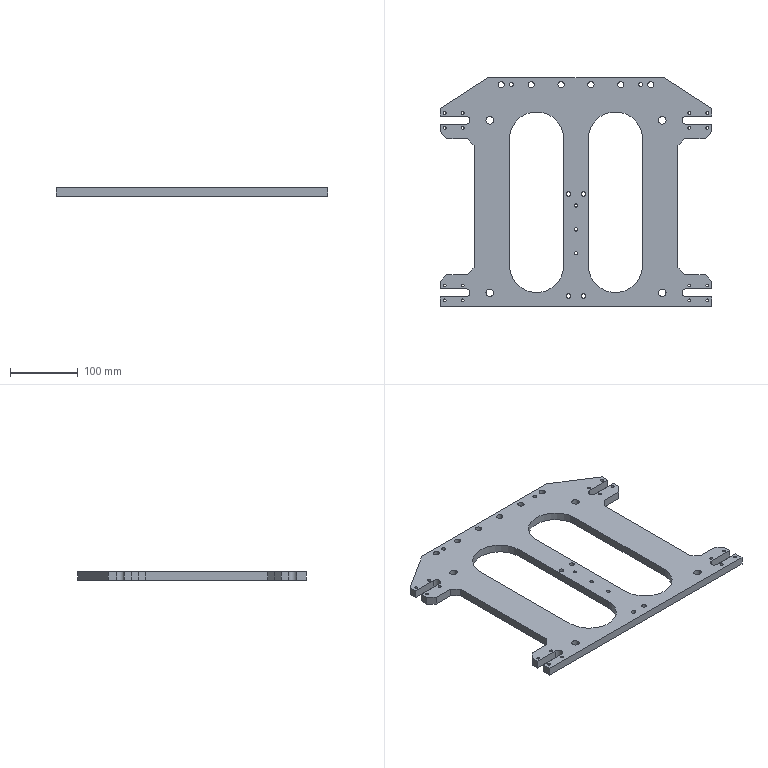NC program | NX | posted with a generic post | part box 400 x 336 x 12 mm
Lines 2735 to 3199 of 3199:
(ZLEVEL_PROFILE_COPY , TOOL : D10JING)
N5420 T09 M6
N5422 G54
N5424 G17 G0 G90 X-207.793 Y129.266 S5000 M3
N5426 G43 Z80. H9
N5428 Z-9.
N5430 G94 G1 Z-12. F1200.
N5432 X-203.703 Y127.158
N5434 G3 X-202.704 Y127.206 R1.
N5436 G1 X-132.704 Y172.206
N5438 G2 X-130. Y173. R5.
N5440 G1 X130.
N5442 G2 X132.704 Y172.206 R5.
N5444 G1 X202.704 Y127.206
N5446 G3 X203.703 Y127.158 R1.
N5448 G1 X207.793 Y129.266
N5450 Z-9.
N5452 G0 Z80.
N5454 X203.167 Y-177.485
N5456 Z-9.
N5458 G1 Z-12.
N5460 X200.866 Y-173.5
N5462 G3 X200. Y-173. R1.
N5464 G1 X-200.
N5466 G3 X-200.866 Y-173.5 R1.
N5468 G1 X-203.167 Y-177.485
N5470 Z-9.
N5472 G0 Z80.
N5474 M5
(ZLEVEL_PROFILE_COPY_COPY_1 , TOOL : D6)
N5476 T06 M6
N5478 G54
N5480 G17 G0 G90 X-94.939 Y78.263 S5000 M3
N5482 G43 Z80. H6
N5484 Z-8.9
N5486 G94 G1 Z-11.9 F1200.
N5488 G3 X-95. Y78. R0.6
N5490 G1 Y-108.
N5492 G3 X-58. Y-145. R37.
N5494 X-21. Y-108. R37.
N5496 G1 Y78.
N5498 G3 X-58. Y115. R37.
N5500 X-95. Y78. R37.
N5502 X-94.94 Y77.738 R0.6
N5504 G1 Z-8.9
N5506 G0 Z80.
N5508 X94.939 Y-108.263
N5510 Z-8.9
N5512 G1 Z-11.9
N5514 G3 X95. Y-108. R0.6
N5516 G1 Y78.
N5518 G3 X58. Y115. R37.
N5520 X21. Y78. R37.
N5522 G1 Y-108.
N5524 G3 X58. Y-145. R37.
N5526 X95. Y-108. R37.
N5528 X94.94 Y-107.738 R0.6
N5530 G1 Z-8.9
N5532 G0 Z80.
N5534 M5
(ZLEVEL_PROFILE_COPY_COPY , TOOL : D6A45)
N5536 T07 M6
N5538 G54
N5540 G17 G0 G90 X-194.483 Y116.5 S7500 M3
N5542 G43 Z80. H7
N5544 Z3.
N5546 G94 G1 Z-1. F1200.
N5548 G3 X-193.3 Y115.317 R1.183
N5550 X-194.483 Y116.5 R-1.183
N5552 X-194.183 Y115.98 R0.6
N5554 G1 Z2.
N5556 G0 Z80.
N5558 X-94.753 Y158.848
N5560 Z2.
N5562 G1 Z-1.
N5564 X-94.48 Y159.783
N5566 G3 X-95. Y160.083 R0.6
N5568 X-97.083 Y158. R2.083
N5570 X-95. Y160.083 R-2.083
N5572 X-95.52 Y159.783 R0.6
N5574 G1 X-95.247 Y158.848
N5576 Z2.
N5578 G0 Z80.
N5580 X95.247
N5582 Z2.
N5584 G1 Z-1.
N5586 X95.52 Y159.783
N5588 G3 X95. Y160.083 R0.6
N5590 X92.917 Y158. R2.083
N5592 X95. Y160.083 R-2.083
N5594 X94.48 Y159.783 R0.6
N5596 G1 X94.753 Y158.848
N5598 Z2.
N5600 G0 Z80.
N5602 X128.157 Y108.679
N5604 Z2.
N5606 G1 Z-1.
N5608 X127.52 Y109.783
N5610 G3 X127. Y110.083 R0.6
N5612 X122.417 Y105.5 R4.583
N5614 X127. Y110.083 R-4.583
N5616 X126.48 Y109.783 R0.6
N5618 G1 X125.843 Y108.679
N5620 Z2.
N5622 G0 Z80.
N5624 X-125.843
N5626 Z2.
N5628 G1 Z-1.
N5630 X-126.48 Y109.783
N5632 G3 X-127. Y110.083 R0.6
N5634 X-131.583 Y105.5 R4.583
N5636 X-127. Y110.083 R-4.583
N5638 X-127.52 Y109.783 R0.6
N5640 G1 X-128.157 Y108.679
N5642 Z2.
N5644 G0 Z80.
N5646 X194.483 Y94.5
N5648 Z3.
N5650 G1 Z-1.
N5652 G3 X193.3 Y95.683 R1.183
N5654 X194.483 Y94.5 R-1.183
N5656 X194.183 Y95.02 R0.6
N5658 G1 Z2.
N5660 G0 Z80.
N5662 X167.883 Y94.5
N5664 Z3.
N5666 G1 Z-1.
N5668 G3 X166.7 Y95.683 R1.183
N5670 X167.883 Y94.5 R-1.183
N5672 X167.583 Y95.02 R0.6
N5674 G1 Z2.
N5676 G0 Z80.
N5678 X-167.883 Y94.5
N5680 Z3.
N5682 G1 Z-1.
N5684 G3 X-166.7 Y93.317 R1.183
N5686 X-167.883 Y94.5 R-1.183
N5688 X-167.583 Y93.98 R0.6
N5690 G1 Z2.
N5692 G0 Z80.
N5694 X-194.483 Y94.5
N5696 Z3.
N5698 G1 Z-1.
N5700 G3 X-193.3 Y93.317 R1.183
N5702 X-194.483 Y94.5 R-1.183
N5704 X-194.183 Y93.98 R0.6
N5706 G1 Z2.
N5708 G0 Z80.
N5710 X111.24 Y160.035
N5712 Z2.
N5714 G1 Z-1.
N5716 X110.52 Y161.283
N5718 G3 X110. Y161.583 R0.6
N5720 X106.417 Y158. R3.583
N5722 X110. Y161.583 R-3.583
N5724 X109.48 Y161.283 R0.6
N5726 G1 X108.76 Y160.035
N5728 Z2.
N5730 G0 Z80.
N5732 X67.24
N5734 Z2.
N5736 G1 Z-1.
N5738 X66.52 Y161.283
N5740 G3 X66. Y161.583 R0.6
N5742 X62.417 Y158. R3.583
N5744 X66. Y161.583 R-3.583
N5746 X65.48 Y161.283 R0.6
N5748 G1 X64.76 Y160.035
N5750 Z2.
N5752 G0 Z80.
N5754 X10.614 Y-4.148
N5756 Z2.
N5758 G1 Z-1.
N5760 X10.38 Y-5.083
N5762 G3 X10.9 Y-5.383 R0.6
N5764 X13.283 Y-3. R2.383
N5766 X10.9 Y-5.383 R-2.383
N5768 X11.42 Y-5.083 R0.6
N5770 G1 X11.186 Y-4.148
N5772 Z2.
N5774 G0 Z80.
N5776 X-11.186
N5778 Z2.
N5780 G1 Z-1.
N5782 X-11.42 Y-5.083
N5784 G3 X-10.9 Y-5.383 R0.6
N5786 X-8.517 Y-3. R2.383
N5788 X-10.9 Y-5.383 R-2.383
N5790 X-10.38 Y-5.083 R0.6
N5792 G1 X-10.614 Y-4.148
N5794 Z2.
N5796 G0 Z80.
N5798 X-0.144 Y-20.355
N5800 Z2.
N5802 G1 Z-1.
N5804 X-0.52 Y-21.283
N5806 G3 X0. Y-21.583 R0.6
N5808 X1.583 Y-20. R1.583
N5810 X0. Y-21.583 R-1.583
N5812 X0.52 Y-21.283 R0.6
N5814 G1 X0.144 Y-20.355
N5816 Z2.
N5818 G0 Z80.
N5820 X-0.144 Y-55.355
N5822 Z2.
N5824 G1 Z-1.
N5826 X-0.52 Y-56.283
N5828 G3 X0. Y-56.583 R0.6
N5830 X1.583 Y-55. R1.583
N5832 X0. Y-56.583 R-1.583
N5834 X0.52 Y-56.283 R0.6
N5836 G1 X0.144 Y-55.355
N5838 Z2.
N5840 G0 Z80.
N5842 X-0.144 Y-90.355
N5844 Z2.
N5846 G1 Z-1.
N5848 X-0.52 Y-91.283
N5850 G3 X0. Y-91.583 R0.6
N5852 X1.583 Y-90. R1.583
N5854 X0. Y-91.583 R-1.583
N5856 X0.52 Y-91.283 R0.6
N5858 G1 X0.144 Y-90.355
N5860 Z2.
N5862 G0 Z80.
N5864 X23.24 Y160.035
N5866 Z2.
N5868 G1 Z-1.
N5870 X22.52 Y161.283
N5872 G3 X22. Y161.583 R0.6
N5874 X18.417 Y158. R3.583
N5876 X22. Y161.583 R-3.583
N5878 X21.48 Y161.283 R0.6
N5880 G1 X20.76 Y160.035
N5882 Z2.
N5884 G0 Z80.
N5886 X-20.76
N5888 Z2.
N5890 G1 Z-1.
N5892 X-21.48 Y161.283
N5894 G3 X-22. Y161.583 R0.6
N5896 X-25.583 Y158. R3.583
N5898 X-22. Y161.583 R-3.583
N5900 X-22.52 Y161.283 R0.6
N5902 G1 X-23.24 Y160.035
N5904 Z2.
N5906 G0 Z80.
N5908 X95.883 Y-16.039
N5910 Z2.
N5912 G1 Z-1.
N5914 X96.783 Y-15.52
N5916 G3 X97.083 Y-15. R0.6
N5918 G1 Y78.
N5920 G3 X58. Y117.083 R39.083
N5922 X18.917 Y78. R39.083
N5924 G1 Y-108.
N5926 G3 X58. Y-147.083 R39.083
N5928 X97.083 Y-108. R39.083
N5930 G1 Y-15.
N5932 G3 X96.783 Y-14.48 R0.6
N5934 G1 X95.883 Y-13.961
N5936 Z2.
N5938 G0 Z80.
N5940 X-95.883
N5942 Z2.
N5944 G1 Z-1.
N5946 X-96.783 Y-14.48
N5948 G3 X-97.083 Y-15. R0.6
N5950 G1 Y-108.
N5952 G3 X-58. Y-147.083 R39.083
N5954 X-18.917 Y-108. R39.083
N5956 G1 Y78.
N5958 G3 X-58. Y117.083 R39.083
N5960 X-97.083 Y78. R39.083
N5962 G1 Y-15.
N5964 G3 X-96.783 Y-15.52 R0.6
N5966 G1 X-95.883 Y-16.039
N5968 Z2.
N5970 G0 Z80.
N5972 X194.483 Y-137.5
N5974 Z3.
N5976 G1 Z-1.
N5978 G3 X193.3 Y-136.317 R1.183
N5980 X194.483 Y-137.5 R-1.183
N5982 X194.183 Y-136.98 R0.6
N5984 G1 Z2.
N5986 G0 Z80.
N5988 X166.7 Y-138.683
N5990 Z3.
N5992 G1 Z-1.
N5994 G3 X167.883 Y-137.5 R1.183
N5996 X166.7 Y-138.683 R-1.183
N5998 X167.22 Y-138.383 R0.6
N6000 G1 Z2.
N6002 G0 Z80.
N6004 X-166.7 Y-138.683
N6006 Z3.
N6008 G1 Z-1.
N6010 G3 X-165.517 Y-137.5 R1.183
N6012 X-166.7 Y-138.683 R-1.183
N6014 X-166.18 Y-138.383 R0.6
N6016 G1 Z2.
N6018 G0 Z80.
N6020 X-194.483 Y-137.5
N6022 Z3.
N6024 G1 Z-1.
N6026 G3 X-193.3 Y-138.683 R1.183
N6028 X-194.483 Y-137.5 R-1.183
N6030 X-194.183 Y-138.02 R0.6
N6032 G1 Z2.
N6034 G0 Z80.
N6036 X-64.76 Y160.035
N6038 Z2.
N6040 G1 Z-1.
N6042 X-65.48 Y161.283
N6044 G3 X-66. Y161.583 R0.6
N6046 X-69.583 Y158. R3.583
N6048 X-66. Y161.583 R-3.583
N6050 X-66.52 Y161.283 R0.6
N6052 G1 X-67.24 Y160.035
N6054 Z2.
N6056 G0 Z80.
N6058 X-108.76
N6060 Z2.
N6062 G1 Z-1.
N6064 X-109.48 Y161.283
N6066 G3 X-110. Y161.583 R0.6
N6068 X-113.583 Y158. R3.583
N6070 X-110. Y161.583 R-3.583
N6072 X-110.52 Y161.283 R0.6
N6074 G1 X-111.24 Y160.035
N6076 Z2.
N6078 G0 Z80.
N6080 X125.843 Y-151.679
N6082 Z2.
N6084 G1 Z-1.
N6086 X126.48 Y-152.783
N6088 G3 X127. Y-153.083 R0.6
N6090 X131.583 Y-148.5 R4.583
N6092 X127. Y-153.083 R-4.583
N6094 X127.52 Y-152.783 R0.6
N6096 G1 X128.157 Y-151.679
N6098 Z2.
N6100 G0 Z80.
N6102 X-128.157
N6104 Z2.
N6106 G1 Z-1.
N6108 X-127.52 Y-152.783
N6110 G3 X-127. Y-153.083 R0.6
N6112 X-122.417 Y-148.5 R4.583
N6114 X-127. Y-153.083 R-4.583
N6116 X-126.48 Y-152.783 R0.6
N6118 G1 X-125.843 Y-151.679
N6120 Z2.
N6122 G0 Z80.
N6124 X194.483 Y116.5
N6126 Z3.
N6128 G1 Z-1.
N6130 G3 X193.3 Y117.683 R1.183
N6132 X194.483 Y116.5 R-1.183
N6134 X194.183 Y117.02 R0.6
N6136 G1 Z2.
N6138 G0 Z80.
N6140 X167.883 Y116.5
N6142 Z3.
N6144 G1 Z-1.
N6146 G3 X166.7 Y117.683 R1.183
N6148 X167.883 Y116.5 R-1.183
N6150 X167.583 Y117.02 R0.6
N6152 G1 Z2.
N6154 G0 Z80.
N6156 X10.614 Y-154.148
N6158 Z2.
N6160 G1 Z-1.
N6162 X10.38 Y-155.083
N6164 G3 X10.9 Y-155.383 R0.6
N6166 X13.283 Y-153. R2.383
N6168 X10.9 Y-155.383 R-2.383
N6170 X11.42 Y-155.083 R0.6
N6172 G1 X11.186 Y-154.148
N6174 Z2.
N6176 G0 Z80.
N6178 X-11.186
N6180 Z2.
N6182 G1 Z-1.
N6184 X-11.42 Y-155.083
N6186 G3 X-10.9 Y-155.383 R0.6
N6188 X-8.517 Y-153. R2.383
N6190 X-10.9 Y-155.383 R-2.383
N6192 X-10.38 Y-155.083 R0.6
N6194 G1 X-10.614 Y-154.148
N6196 Z2.
N6198 G0 Z80.
N6200 X194.483 Y-159.5
N6202 Z3.
N6204 G1 Z-1.
N6206 G3 X193.3 Y-158.317 R1.183
N6208 X194.483 Y-159.5 R-1.183
N6210 X194.183 Y-158.98 R0.6
N6212 G1 Z2.
N6214 G0 Z80.
N6216 X166.7 Y-160.683
N6218 Z3.
N6220 G1 Z-1.
N6222 G3 X167.883 Y-159.5 R1.183
N6224 X166.7 Y-160.683 R-1.183
N6226 X167.22 Y-160.383 R0.6
N6228 G1 Z2.
N6230 G0 Z80.
N6232 X-166.7 Y-160.683
N6234 Z3.
N6236 G1 Z-1.
N6238 G3 X-165.517 Y-159.5 R1.183
N6240 X-166.7 Y-160.683 R-1.183
N6242 X-166.18 Y-160.383 R0.6
N6244 G1 Z2.
N6246 G0 Z80.
N6248 X-194.483 Y-159.5
N6250 Z3.
N6252 G1 Z-1.
N6254 G3 X-193.3 Y-160.683 R1.183
N6256 X-194.483 Y-159.5 R-1.183
N6258 X-194.183 Y-160.02 R0.6
N6260 G1 Z2.
N6262 G0 Z80.
N6264 X-167.883 Y116.5
N6266 Z3.
N6268 G1 Z-1.
N6270 G3 X-166.7 Y115.317 R1.183
N6272 X-167.883 Y116.5 R-1.183
N6274 X-167.583 Y115.98 R0.6
N6276 G1 Z2.
N6278 G0 Z80.
N6280 X200.073 Y-170.195
N6282 Z2.
N6284 G1 Z-1.
N6286 X199.973 Y-169.396
N6288 G3 X199.611 Y-168.917 R0.6
N6290 G1 X-199.611
N6292 G3 X-199.973 Y-169.396 R0.6
N6294 G1 X-200.073 Y-170.195
N6296 Z2.
N6298 G0 Z80.
N6300 X-201.247 Y124.808
N6302 Z2.
N6304 G1 Z-1.
N6306 X-200.732 Y124.189
N6308 G3 X-200.169 Y123.981 R0.6
N6310 G1 X-130.495 Y168.772
N6312 G2 X-130.001 Y168.917 R0.914
N6314 G1 X130.001
N6316 G2 X130.495 Y168.772 R0.914
N6318 G1 X200.169 Y123.981
N6320 G3 X200.732 Y124.189 R0.6
N6322 G1 X201.247 Y124.808
N6324 Z2.
N6326 G0 Z80.
N6328 M5
N6330 M2